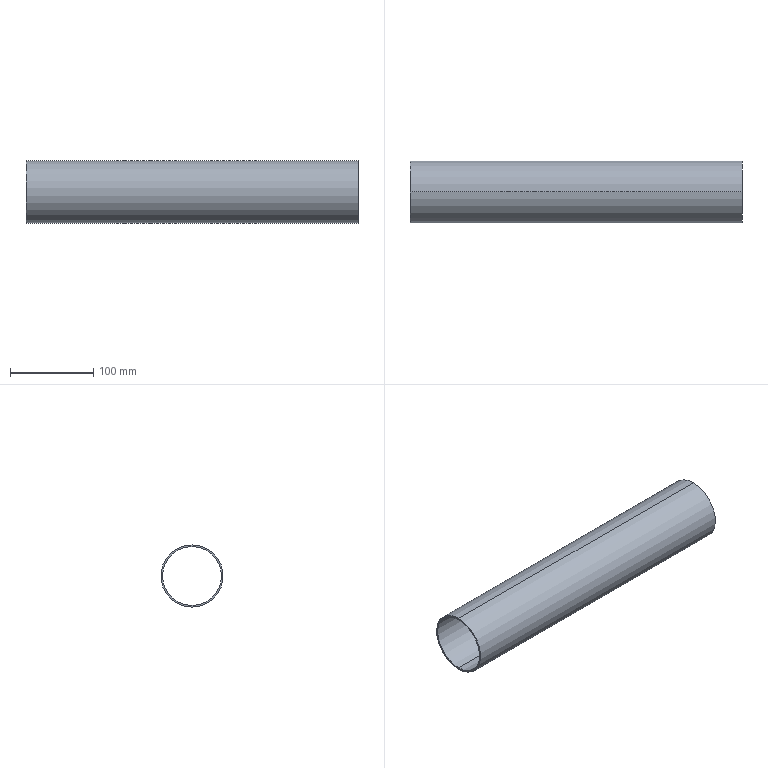Part | STEP file | Flat conveyor mechanism-CN2500x400-107-102 | 1 solid | 6 faces | box 400 x 75 x 75 mm | volume 183469 mm3 | cylinder 4 | plane 2 | commonest cylinder face diameters 71 x2 75 x2
STEP:
#1=CARTESIAN_POINT('',(181.247,0.,37.5));
#2=VERTEX_POINT('',#1);
#3=CARTESIAN_POINT('',(181.247,0.,-37.5));
#4=VERTEX_POINT('',#3);
#5=CARTESIAN_POINT('',(181.247,0.,0.));
#6=DIRECTION('',(-1.,0.,0.));
#7=DIRECTION('',(0.,0.,1.));
#8=AXIS2_PLACEMENT_3D('',#5,#6,#7);
#9=CIRCLE('',#8,37.5);
#10=EDGE_CURVE('',#2,#4,#9,.T.);
#11=ORIENTED_EDGE('',*,*,#10,.T.);
#12=CARTESIAN_POINT('',(-218.753,0.,-37.5));
#13=VERTEX_POINT('',#12);
#14=CARTESIAN_POINT('',(0.,0.,-37.5));
#15=DIRECTION('',(-1.,0.,0.));
#16=VECTOR('',#15,1000.);
#17=LINE('',#14,#16);
#18=EDGE_CURVE('',#4,#13,#17,.T.);
#19=ORIENTED_EDGE('',*,*,#18,.T.);
#20=CARTESIAN_POINT('',(-218.753,0.,37.5));
#21=VERTEX_POINT('',#20);
#22=CARTESIAN_POINT('',(-218.753,0.,0.));
#23=DIRECTION('',(-1.,0.,0.));
#24=DIRECTION('',(0.,0.,1.));
#25=AXIS2_PLACEMENT_3D('',#22,#23,#24);
#26=CIRCLE('',#25,37.5);
#27=EDGE_CURVE('',#21,#13,#26,.T.);
#28=ORIENTED_EDGE('',*,*,#27,.F.);
#29=CARTESIAN_POINT('',(0.,0.,37.5));
#30=DIRECTION('',(-1.,0.,0.));
#31=VECTOR('',#30,1000.);
#32=LINE('',#29,#31);
#33=EDGE_CURVE('',#2,#21,#32,.T.);
#34=ORIENTED_EDGE('',*,*,#33,.F.);
#35=EDGE_LOOP('',(#11,#19,#28,#34));
#36=FACE_OUTER_BOUND('',#35,.T.);
#37=CARTESIAN_POINT('',(0.,0.,0.));
#38=DIRECTION('',(-1.,0.,0.));
#39=DIRECTION('',(0.,0.,1.));
#40=AXIS2_PLACEMENT_3D('',#37,#38,#39);
#41=CYLINDRICAL_SURFACE('',#40,37.5);
#42=ADVANCED_FACE('',(#36),#41,.T.);
#43=CARTESIAN_POINT('',(181.247,0.,-35.5));
#44=VERTEX_POINT('',#43);
#45=CARTESIAN_POINT('',(181.247,0.,35.5));
#46=VERTEX_POINT('',#45);
#47=CARTESIAN_POINT('',(181.247,0.,0.));
#48=DIRECTION('',(-1.,0.,0.));
#49=DIRECTION('',(0.,0.,1.));
#50=AXIS2_PLACEMENT_3D('',#47,#48,#49);
#51=CIRCLE('',#50,35.5);
#52=EDGE_CURVE('',#44,#46,#51,.T.);
#53=ORIENTED_EDGE('',*,*,#52,.F.);
#54=CARTESIAN_POINT('',(-218.753,0.,-35.5));
#55=VERTEX_POINT('',#54);
#56=CARTESIAN_POINT('',(0.,0.,-35.5));
#57=DIRECTION('',(-1.,0.,0.));
#58=VECTOR('',#57,1000.);
#59=LINE('',#56,#58);
#60=EDGE_CURVE('',#44,#55,#59,.T.);
#61=ORIENTED_EDGE('',*,*,#60,.T.);
#62=CARTESIAN_POINT('',(-218.753,0.,35.5));
#63=VERTEX_POINT('',#62);
#64=CARTESIAN_POINT('',(-218.753,0.,0.));
#65=DIRECTION('',(-1.,0.,0.));
#66=DIRECTION('',(0.,0.,1.));
#67=AXIS2_PLACEMENT_3D('',#64,#65,#66);
#68=CIRCLE('',#67,35.5);
#69=EDGE_CURVE('',#55,#63,#68,.T.);
#70=ORIENTED_EDGE('',*,*,#69,.T.);
#71=CARTESIAN_POINT('',(0.,0.,35.5));
#72=DIRECTION('',(-1.,0.,0.));
#73=VECTOR('',#72,1000.);
#74=LINE('',#71,#73);
#75=EDGE_CURVE('',#46,#63,#74,.T.);
#76=ORIENTED_EDGE('',*,*,#75,.F.);
#77=EDGE_LOOP('',(#53,#61,#70,#76));
#78=FACE_OUTER_BOUND('',#77,.T.);
#79=CARTESIAN_POINT('',(0.,0.,0.));
#80=DIRECTION('',(-1.,0.,0.));
#81=DIRECTION('',(0.,0.,1.));
#82=AXIS2_PLACEMENT_3D('',#79,#80,#81);
#83=CYLINDRICAL_SURFACE('',#82,35.5);
#84=ADVANCED_FACE('',(#78),#83,.F.);
#85=CARTESIAN_POINT('',(-218.753,0.,0.));
#86=DIRECTION('',(-1.,0.,0.));
#87=DIRECTION('',(0.,0.,1.));
#88=AXIS2_PLACEMENT_3D('',#85,#86,#87);
#89=CIRCLE('',#88,35.5);
#90=EDGE_CURVE('',#63,#55,#89,.T.);
#91=ORIENTED_EDGE('',*,*,#90,.F.);
#92=ORIENTED_EDGE('',*,*,#69,.F.);
#93=EDGE_LOOP('',(#91,#92));
#94=FACE_BOUND('',#93,.T.);
#95=ORIENTED_EDGE('',*,*,#27,.T.);
#96=CARTESIAN_POINT('',(-218.753,0.,0.));
#97=DIRECTION('',(-1.,0.,0.));
#98=DIRECTION('',(0.,0.,1.));
#99=AXIS2_PLACEMENT_3D('',#96,#97,#98);
#100=CIRCLE('',#99,37.5);
#101=EDGE_CURVE('',#13,#21,#100,.T.);
#102=ORIENTED_EDGE('',*,*,#101,.T.);
#103=EDGE_LOOP('',(#95,#102));
#104=FACE_OUTER_BOUND('',#103,.T.);
#105=CARTESIAN_POINT('',(-218.753,37.5,0.));
#106=DIRECTION('',(1.,0.,0.));
#107=DIRECTION('',(0.,0.,-1.));
#108=AXIS2_PLACEMENT_3D('',#105,#106,#107);
#109=PLANE('',#108);
#110=ADVANCED_FACE('',(#94,#104),#109,.F.);
#111=ORIENTED_EDGE('',*,*,#60,.F.);
#112=CARTESIAN_POINT('',(181.247,0.,0.));
#113=DIRECTION('',(-1.,0.,0.));
#114=DIRECTION('',(0.,0.,1.));
#115=AXIS2_PLACEMENT_3D('',#112,#113,#114);
#116=CIRCLE('',#115,35.5);
#117=EDGE_CURVE('',#46,#44,#116,.T.);
#118=ORIENTED_EDGE('',*,*,#117,.F.);
#119=ORIENTED_EDGE('',*,*,#75,.T.);
#120=ORIENTED_EDGE('',*,*,#90,.T.);
#121=EDGE_LOOP('',(#111,#118,#119,#120));
#122=FACE_OUTER_BOUND('',#121,.T.);
#123=CARTESIAN_POINT('',(0.,0.,0.));
#124=DIRECTION('',(-1.,0.,0.));
#125=DIRECTION('',(0.,0.,1.));
#126=AXIS2_PLACEMENT_3D('',#123,#124,#125);
#127=CYLINDRICAL_SURFACE('',#126,35.5);
#128=ADVANCED_FACE('',(#122),#127,.F.);
#129=ORIENTED_EDGE('',*,*,#10,.F.);
#130=CARTESIAN_POINT('',(181.247,0.,0.));
#131=DIRECTION('',(-1.,0.,0.));
#132=DIRECTION('',(0.,0.,1.));
#133=AXIS2_PLACEMENT_3D('',#130,#131,#132);
#134=CIRCLE('',#133,37.5);
#135=EDGE_CURVE('',#4,#2,#134,.T.);
#136=ORIENTED_EDGE('',*,*,#135,.F.);
#137=EDGE_LOOP('',(#129,#136));
#138=FACE_OUTER_BOUND('',#137,.T.);
#139=ORIENTED_EDGE('',*,*,#117,.T.);
#140=ORIENTED_EDGE('',*,*,#52,.T.);
#141=EDGE_LOOP('',(#139,#140));
#142=FACE_BOUND('',#141,.T.);
#143=CARTESIAN_POINT('',(181.247,35.5,0.));
#144=DIRECTION('',(-1.,0.,0.));
#145=DIRECTION('',(0.,0.,1.));
#146=AXIS2_PLACEMENT_3D('',#143,#144,#145);
#147=PLANE('',#146);
#148=ADVANCED_FACE('',(#138,#142),#147,.F.);
#149=ORIENTED_EDGE('',*,*,#18,.F.);
#150=ORIENTED_EDGE('',*,*,#135,.T.);
#151=ORIENTED_EDGE('',*,*,#33,.T.);
#152=ORIENTED_EDGE('',*,*,#101,.F.);
#153=EDGE_LOOP('',(#149,#150,#151,#152));
#154=FACE_OUTER_BOUND('',#153,.T.);
#155=CARTESIAN_POINT('',(0.,0.,0.));
#156=DIRECTION('',(-1.,0.,0.));
#157=DIRECTION('',(0.,0.,1.));
#158=AXIS2_PLACEMENT_3D('',#155,#156,#157);
#159=CYLINDRICAL_SURFACE('',#158,37.5);
#160=ADVANCED_FACE('',(#154),#159,.T.);
#161=CLOSED_SHELL('',(#42,#84,#110,#128,#148,#160));
#162=MANIFOLD_SOLID_BREP('',#161);
#163=CARTESIAN_POINT('',(0.,0.,0.));
#164=DIRECTION('',(0.,0.,1.));
#165=DIRECTION('',(1.,0.,0.));
#166=AXIS2_PLACEMENT_3D('',#163,#164,#165);
#167=(LENGTH_UNIT()NAMED_UNIT(*)SI_UNIT(.MILLI.,.METRE.));
#168=UNCERTAINTY_MEASURE_WITH_UNIT(LENGTH_MEASURE(0.00001),#167,'','');
#169=(NAMED_UNIT(*)PLANE_ANGLE_UNIT()SI_UNIT($,.RADIAN.));
#170=(NAMED_UNIT(*)SI_UNIT($,.STERADIAN.)SOLID_ANGLE_UNIT());
#171=(GEOMETRIC_REPRESENTATION_CONTEXT(3)GLOBAL_UNCERTAINTY_ASSIGNED_CONTEXT((#168))GLOBAL_UNIT_ASSIGNED_CONTEXT((#167,#169,#170))REPRESENTATION_CONTEXT('',''));
#172=ADVANCED_BREP_SHAPE_REPRESENTATION('',(#162,#166),#171);